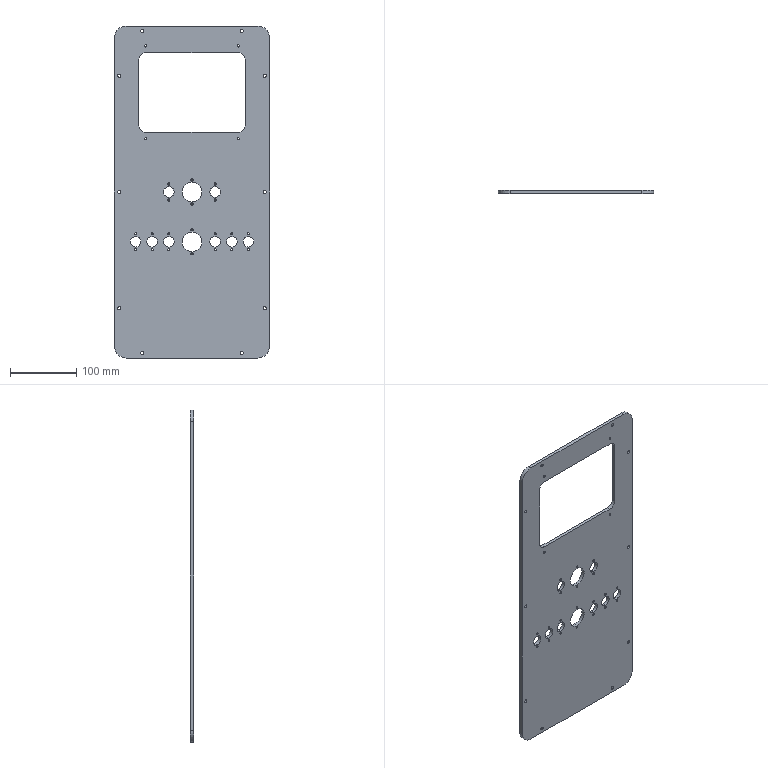Part | SolidWorks | features 3DProfileFeature 5, HoleWzd 5, ICE 3, Fillet 2, Extrusion 1 | 1 solid | 106 faces | box 234 x 5 x 500 mm | volume 471230 mm3 | cylinder 96 | plane 10 | commonest cylinder face diameters 3.3 x48 4.8 x20 16 x16 20 x4 29.5 x4 36 x4